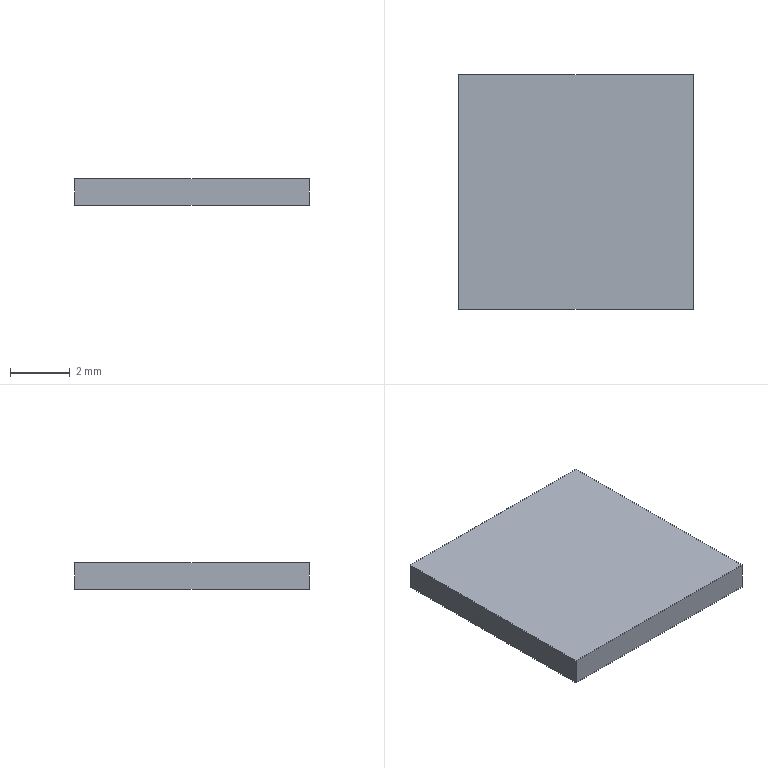Part | Creo | 1 solid | 6 faces | box 7.835 x 7.835 x 0.8999 mm | volume 55.244 mm3 | plane 6
STEP:
#1=CARTESIAN_POINT('',(0.,0.,0.));
#2=DIRECTION('',(0.,0.,1.));
#3=DIRECTION('',(1.,0.,0.));
#4=AXIS2_PLACEMENT_3D('',#1,#2,#3);
#5=CARTESIAN_POINT('',(-3.918,-3.918,0.));
#6=VERTEX_POINT('',#5);
#7=CARTESIAN_POINT('',(3.918,-3.918,0.));
#8=VERTEX_POINT('',#7);
#9=CARTESIAN_POINT('',(-3.918,-3.918,0.));
#10=DIRECTION('',(1.,0.,0.));
#11=VECTOR('',#10,7.835);
#12=LINE('',#9,#11);
#13=EDGE_CURVE('',#6,#8,#12,.T.);
#14=ORIENTED_EDGE('',*,*,#13,.T.);
#15=CARTESIAN_POINT('',(3.918,3.918,0.));
#16=VERTEX_POINT('',#15);
#17=CARTESIAN_POINT('',(3.918,-3.918,0.));
#18=DIRECTION('',(0.,1.,0.));
#19=VECTOR('',#18,7.835);
#20=LINE('',#17,#19);
#21=EDGE_CURVE('',#8,#16,#20,.T.);
#22=ORIENTED_EDGE('',*,*,#21,.T.);
#23=CARTESIAN_POINT('',(-3.918,3.918,0.));
#24=VERTEX_POINT('',#23);
#25=CARTESIAN_POINT('',(3.918,3.918,0.));
#26=DIRECTION('',(-1.,0.,0.));
#27=VECTOR('',#26,7.835);
#28=LINE('',#25,#27);
#29=EDGE_CURVE('',#16,#24,#28,.T.);
#30=ORIENTED_EDGE('',*,*,#29,.T.);
#31=CARTESIAN_POINT('',(-3.918,3.918,0.));
#32=DIRECTION('',(0.,-1.,0.));
#33=VECTOR('',#32,7.835);
#34=LINE('',#31,#33);
#35=EDGE_CURVE('',#24,#6,#34,.T.);
#36=ORIENTED_EDGE('',*,*,#35,.T.);
#37=EDGE_LOOP('',(#14,#22,#30,#36));
#38=FACE_OUTER_BOUND('',#37,.F.);
#39=CARTESIAN_POINT('',(0.,0.,0.));
#40=DIRECTION('',(0.,0.,1.));
#41=DIRECTION('',(1.,0.,0.));
#42=AXIS2_PLACEMENT_3D('',#39,#40,#41);
#43=PLANE('',#42);
#44=ADVANCED_FACE('',(#38),#43,.F.);
#45=ORIENTED_EDGE('',*,*,#13,.F.);
#46=CARTESIAN_POINT('',(-3.918,-3.918,0.8999));
#47=VERTEX_POINT('',#46);
#48=CARTESIAN_POINT('',(-3.918,-3.918,0.));
#49=DIRECTION('',(0.,0.,1.));
#50=VECTOR('',#49,0.8999);
#51=LINE('',#48,#50);
#52=EDGE_CURVE('',#6,#47,#51,.T.);
#53=ORIENTED_EDGE('',*,*,#52,.T.);
#54=CARTESIAN_POINT('',(3.918,-3.918,0.8999));
#55=VERTEX_POINT('',#54);
#56=CARTESIAN_POINT('',(-3.918,-3.918,0.8999));
#57=DIRECTION('',(1.,0.,0.));
#58=VECTOR('',#57,7.835);
#59=LINE('',#56,#58);
#60=EDGE_CURVE('',#47,#55,#59,.T.);
#61=ORIENTED_EDGE('',*,*,#60,.T.);
#62=CARTESIAN_POINT('',(3.918,-3.918,0.));
#63=DIRECTION('',(0.,0.,1.));
#64=VECTOR('',#63,0.8999);
#65=LINE('',#62,#64);
#66=EDGE_CURVE('',#8,#55,#65,.T.);
#67=ORIENTED_EDGE('',*,*,#66,.F.);
#68=EDGE_LOOP('',(#45,#53,#61,#67));
#69=FACE_OUTER_BOUND('',#68,.F.);
#70=CARTESIAN_POINT('',(-3.918,-3.918,0.));
#71=DIRECTION('',(0.,-1.,0.));
#72=DIRECTION('',(1.,0.,0.));
#73=AXIS2_PLACEMENT_3D('',#70,#71,#72);
#74=PLANE('',#73);
#75=ADVANCED_FACE('',(#69),#74,.T.);
#76=ORIENTED_EDGE('',*,*,#35,.F.);
#77=CARTESIAN_POINT('',(-3.918,3.918,0.8999));
#78=VERTEX_POINT('',#77);
#79=CARTESIAN_POINT('',(-3.918,3.918,0.));
#80=DIRECTION('',(0.,0.,1.));
#81=VECTOR('',#80,0.8999);
#82=LINE('',#79,#81);
#83=EDGE_CURVE('',#24,#78,#82,.T.);
#84=ORIENTED_EDGE('',*,*,#83,.T.);
#85=CARTESIAN_POINT('',(-3.918,3.918,0.8999));
#86=DIRECTION('',(0.,-1.,0.));
#87=VECTOR('',#86,7.835);
#88=LINE('',#85,#87);
#89=EDGE_CURVE('',#78,#47,#88,.T.);
#90=ORIENTED_EDGE('',*,*,#89,.T.);
#91=ORIENTED_EDGE('',*,*,#52,.F.);
#92=EDGE_LOOP('',(#76,#84,#90,#91));
#93=FACE_OUTER_BOUND('',#92,.F.);
#94=CARTESIAN_POINT('',(-3.918,3.918,0.));
#95=DIRECTION('',(-1.,0.,0.));
#96=DIRECTION('',(0.,-1.,0.));
#97=AXIS2_PLACEMENT_3D('',#94,#95,#96);
#98=PLANE('',#97);
#99=ADVANCED_FACE('',(#93),#98,.T.);
#100=ORIENTED_EDGE('',*,*,#29,.F.);
#101=CARTESIAN_POINT('',(3.918,3.918,0.8999));
#102=VERTEX_POINT('',#101);
#103=CARTESIAN_POINT('',(3.918,3.918,0.));
#104=DIRECTION('',(0.,0.,1.));
#105=VECTOR('',#104,0.8999);
#106=LINE('',#103,#105);
#107=EDGE_CURVE('',#16,#102,#106,.T.);
#108=ORIENTED_EDGE('',*,*,#107,.T.);
#109=CARTESIAN_POINT('',(3.918,3.918,0.8999));
#110=DIRECTION('',(-1.,0.,0.));
#111=VECTOR('',#110,7.835);
#112=LINE('',#109,#111);
#113=EDGE_CURVE('',#102,#78,#112,.T.);
#114=ORIENTED_EDGE('',*,*,#113,.T.);
#115=ORIENTED_EDGE('',*,*,#83,.F.);
#116=EDGE_LOOP('',(#100,#108,#114,#115));
#117=FACE_OUTER_BOUND('',#116,.F.);
#118=CARTESIAN_POINT('',(3.918,3.918,0.));
#119=DIRECTION('',(0.,1.,0.));
#120=DIRECTION('',(-1.,0.,0.));
#121=AXIS2_PLACEMENT_3D('',#118,#119,#120);
#122=PLANE('',#121);
#123=ADVANCED_FACE('',(#117),#122,.T.);
#124=ORIENTED_EDGE('',*,*,#21,.F.);
#125=ORIENTED_EDGE('',*,*,#66,.T.);
#126=CARTESIAN_POINT('',(3.918,-3.918,0.8999));
#127=DIRECTION('',(0.,1.,0.));
#128=VECTOR('',#127,7.835);
#129=LINE('',#126,#128);
#130=EDGE_CURVE('',#55,#102,#129,.T.);
#131=ORIENTED_EDGE('',*,*,#130,.T.);
#132=ORIENTED_EDGE('',*,*,#107,.F.);
#133=EDGE_LOOP('',(#124,#125,#131,#132));
#134=FACE_OUTER_BOUND('',#133,.F.);
#135=CARTESIAN_POINT('',(3.918,-3.918,0.));
#136=DIRECTION('',(1.,0.,0.));
#137=DIRECTION('',(0.,1.,0.));
#138=AXIS2_PLACEMENT_3D('',#135,#136,#137);
#139=PLANE('',#138);
#140=ADVANCED_FACE('',(#134),#139,.T.);
#141=ORIENTED_EDGE('',*,*,#60,.F.);
#142=ORIENTED_EDGE('',*,*,#89,.F.);
#143=ORIENTED_EDGE('',*,*,#113,.F.);
#144=ORIENTED_EDGE('',*,*,#130,.F.);
#145=EDGE_LOOP('',(#141,#142,#143,#144));
#146=FACE_OUTER_BOUND('',#145,.F.);
#147=CARTESIAN_POINT('',(0.,0.,0.8999));
#148=DIRECTION('',(0.,0.,1.));
#149=DIRECTION('',(1.,0.,0.));
#150=AXIS2_PLACEMENT_3D('',#147,#148,#149);
#151=PLANE('',#150);
#152=ADVANCED_FACE('',(#146),#151,.T.);
#153=CLOSED_SHELL('',(#44,#75,#99,#123,#140,#152));
#154=MANIFOLD_SOLID_BREP('',#153);
#155=(LENGTH_UNIT()NAMED_UNIT(*)SI_UNIT(.MILLI.,.METRE.));
#156=UNCERTAINTY_MEASURE_WITH_UNIT(LENGTH_MEASURE(0.001112),#155,'','');
#157=(NAMED_UNIT(*)PLANE_ANGLE_UNIT()SI_UNIT($,.RADIAN.));
#158=PLANE_ANGLE_MEASURE_WITH_UNIT(PLANE_ANGLE_MEASURE(0.01745),#157);
#159=(CONVERSION_BASED_UNIT('DEGREE',#158)NAMED_UNIT(*)PLANE_ANGLE_UNIT());
#160=(NAMED_UNIT(*)SI_UNIT($,.STERADIAN.)SOLID_ANGLE_UNIT());
#161=(GEOMETRIC_REPRESENTATION_CONTEXT(3)GLOBAL_UNCERTAINTY_ASSIGNED_CONTEXT((#156))GLOBAL_UNIT_ASSIGNED_CONTEXT((#155,#159,#160))REPRESENTATION_CONTEXT('',''));
#162=ADVANCED_BREP_SHAPE_REPRESENTATION('',(#4,#154),#161);